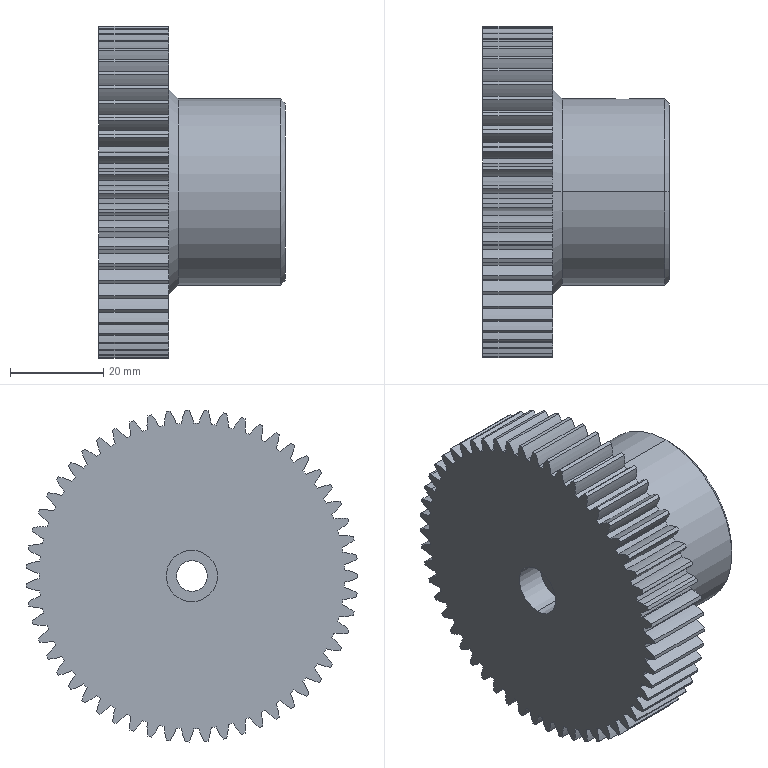Part | SolidWorks | features Chamfer 3, ICE 3, HoleWzd 2, BaseBody 1 | 1 solid | 250 faces | box 40 x 71.213 x 71.239 mm | volume 76769 mm3 | cylinder 235 | plane 8 | cone 7 | commonest cylinder face diameters 27.5 x114 65.623 x55 71.25 x55 19 x3 4.2 x2 6.6 x2